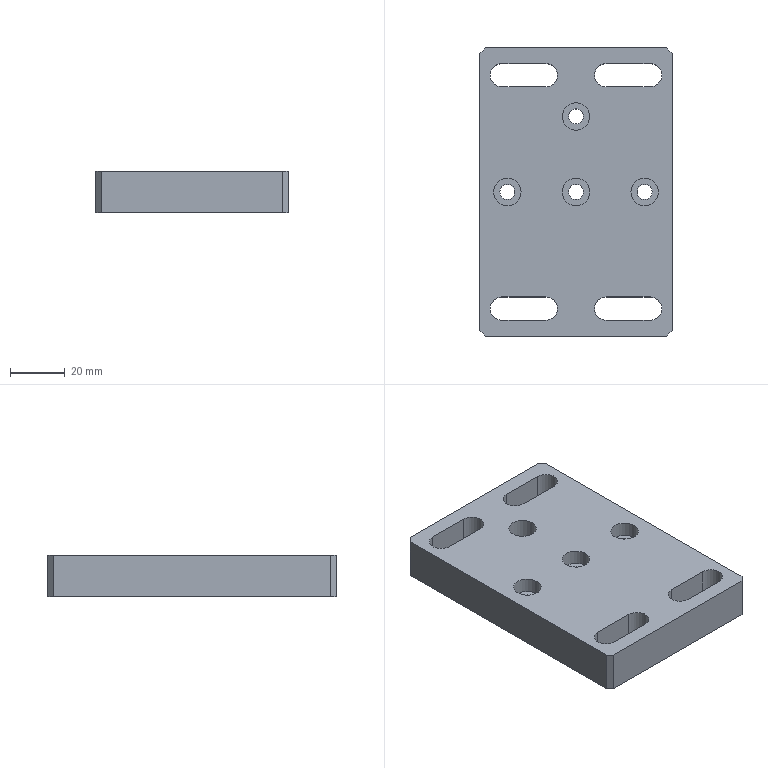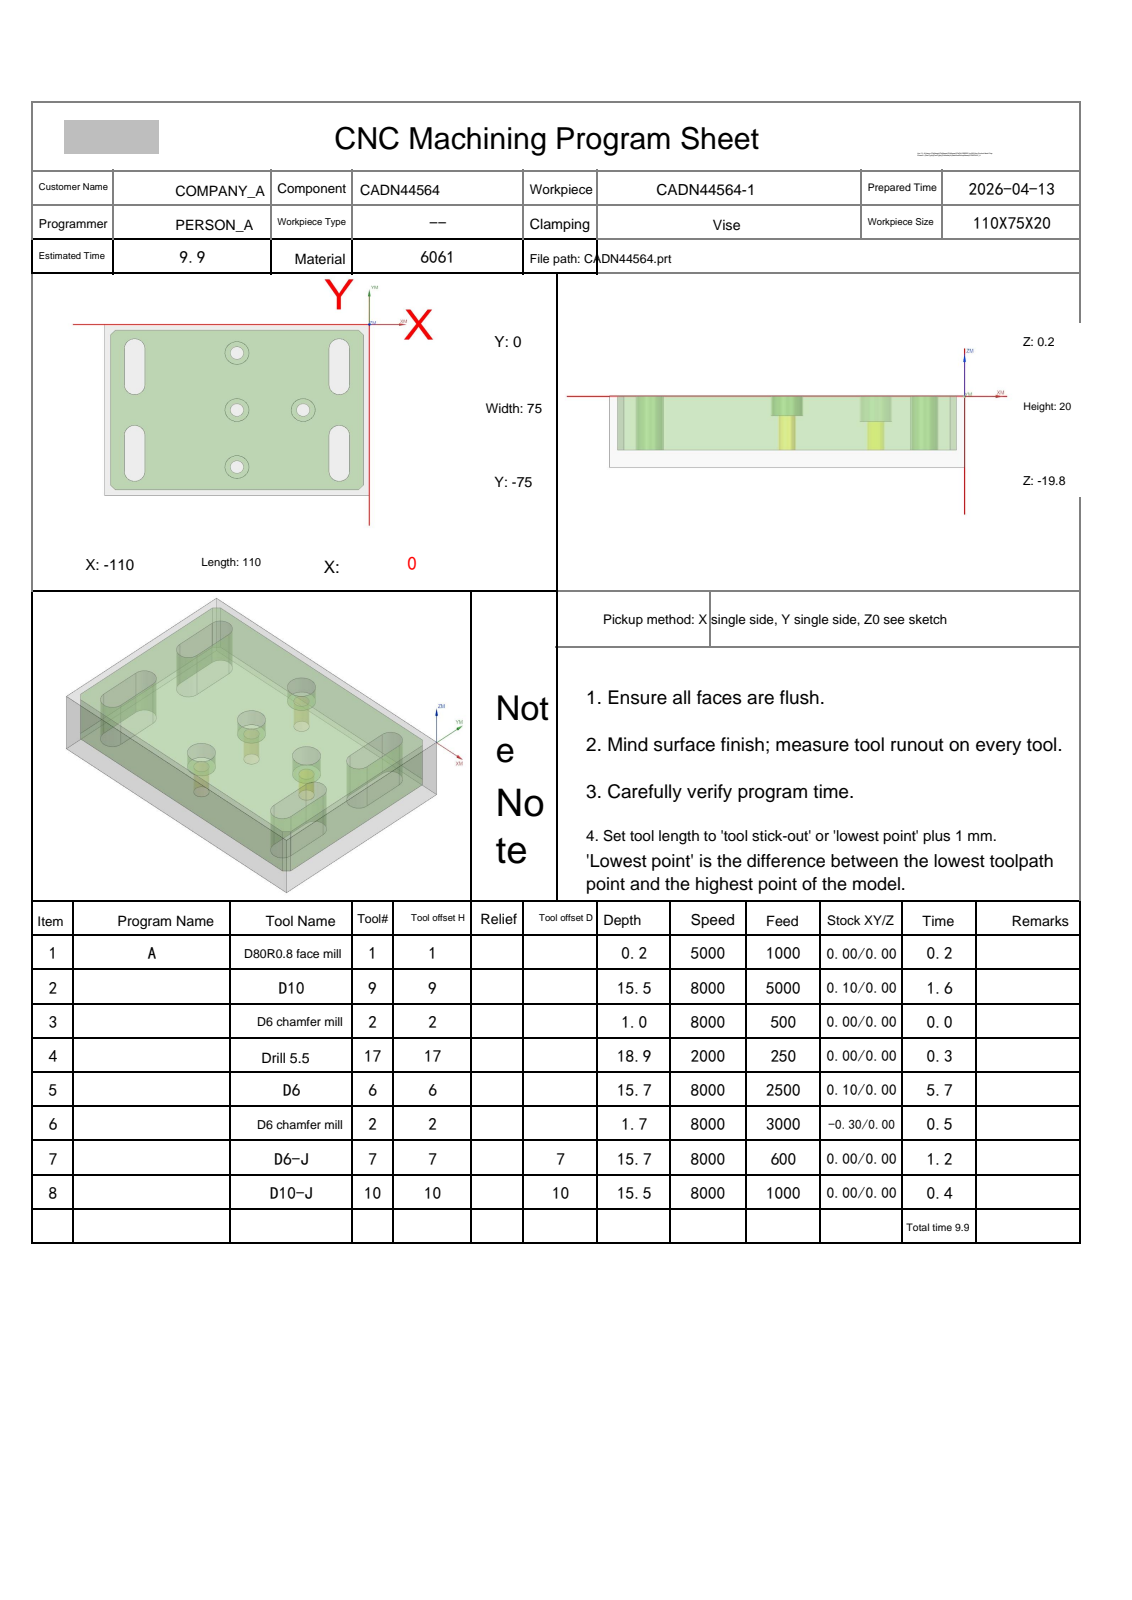NC program | NX | posted by the shop | part box 70 x 105 x 15 mm
Lines 2582 to 3183 of 3183:
N6 T02 M06
(D6 chamfer mill  D=6. R=0. H=02 ce=0.00 di=0.00)
G00 G90 G54 X-54.75 Y-74.628 M03 S8000
G43 H02 Z20.
M08
Z2.099
G01 Z-1.5 F3000.
G03 X-54.67 Y-74.328 I-.52 J.3
X-54.97 Y-73.808 I-.6 J0.0
G01 X-55. Y-73.8
X-105.5
X-105.754 Y-73.775
X-105.997 Y-73.701
X-106.222 Y-73.581
X-106.419 Y-73.419
X-108.419 Y-71.419
X-108.581 Y-71.222
X-108.701 Y-70.997
X-108.775 Y-70.754
X-108.8 Y-70.5
Y-4.5
X-108.775 Y-4.246
X-108.701 Y-4.003
X-108.581 Y-3.778
X-108.419 Y-3.581
X-106.419 Y-1.581
X-106.222 Y-1.419
X-105.997 Y-1.299
X-105.754 Y-1.225
X-105.5 Y-1.2
X-4.5
X-4.246 Y-1.225
X-4.003 Y-1.299
X-3.778 Y-1.419
X-3.581 Y-1.581
X-1.581 Y-3.581
X-1.419 Y-3.778
X-1.299 Y-4.003
X-1.225 Y-4.246
X-1.2 Y-4.5
Y-70.5
X-1.225 Y-70.754
X-1.299 Y-70.997
X-1.419 Y-71.222
X-1.581 Y-71.419
X-3.581 Y-73.419
X-3.778 Y-73.581
X-4.003 Y-73.701
X-4.246 Y-73.775
X-4.5 Y-73.8
X-55.
X-55.03 Y-73.808
G03 X-55.33 Y-74.328 I.3 J-.52
X-55.25 Y-74.628 I.6 J0.0
G01 Z2.099
G00 Z20.
X-95.378 Y-56.75
Z2.099
G01 Z-1.5
G03 X-95.078 Y-56.83 I.3 J.52
X-94.558 Y-56.53 I0.0 J.6
G01 X-94.55 Y-56.5
Y-48.5
G03 X-97.5 Y-45.55 I-2.95 J0.0
X-100.45 Y-48.5 I0.0 J-2.95
G01 Y-64.5
G03 X-97.5 Y-67.45 I2.95 J0.0
X-94.55 Y-64.5 I0.0 J2.95
G01 Y-56.5
X-94.558 Y-56.47
G03 X-95.078 Y-56.17 I-.52 J-.3
X-95.378 Y-56.25 I0.0 J-.6
G01 Z2.099
G00 Z20.
Y-18.75
Z2.099
G01 Z-1.5
G03 X-95.078 Y-18.83 I.3 J.52
X-94.558 Y-18.53 I0.0 J.6
G01 X-94.55 Y-18.5
Y-10.5
G03 X-97.5 Y-7.55 I-2.95 J0.0
X-100.45 Y-10.5 I0.0 J-2.95
G01 Y-26.5
G03 X-97.5 Y-29.45 I2.95 J0.0
X-94.55 Y-26.5 I0.0 J2.95
G01 Y-18.5
X-94.558 Y-18.47
G03 X-95.078 Y-18.17 I-.52 J-.3
X-95.378 Y-18.25 I0.0 J-.6
G01 Z2.099
G00 Z20.
X-14.622
Z2.099
G01 Z-1.5
G03 X-14.922 Y-18.17 I-.3 J-.52
X-15.442 Y-18.47 I0.0 J-.6
G01 X-15.45 Y-18.5
Y-26.5
G03 X-12.5 Y-29.45 I2.95 J0.0
X-9.55 Y-26.5 I0.0 J2.95
G01 Y-10.5
G03 X-12.5 Y-7.55 I-2.95 J0.0
X-15.45 Y-10.5 I0.0 J-2.95
G01 Y-18.5
X-15.442 Y-18.53
G03 X-14.922 Y-18.83 I.52 J.3
X-14.622 Y-18.75 I0.0 J.6
G01 Z2.099
G00 Z20.
Y-56.25
Z2.099
G01 Z-1.5
G03 X-14.922 Y-56.17 I-.3 J-.52
X-15.442 Y-56.47 I0.0 J-.6
G01 X-15.45 Y-56.5
Y-64.5
G03 X-12.5 Y-67.45 I2.95 J0.0
X-9.55 Y-64.5 I0.0 J2.95
G01 Y-48.5
G03 X-12.5 Y-45.55 I-2.95 J0.0
X-15.45 Y-48.5 I0.0 J-2.95
G01 Y-56.5
X-15.442 Y-56.53
G03 X-14.922 Y-56.83 I.52 J.3
X-14.622 Y-56.75 I0.0 J.6
G01 Z2.099
G00 Z20.
G00 G90 X-58.386 Y-9.846 M03 S8000
Z20.
Z2.5
G01 X-58.394 Y-9.855 Z2.495 F800.
X-58.644 Y-10.211 Z2.337
X-58.804 Y-10.489 Z2.22
X-58.988 Y-10.883 Z2.062
X-59.13 Y-11.293 Z1.904
X-59.231 Y-11.716 Z1.746
X-59.288 Y-12.146 Z1.588
X-59.302 Y-12.58 Z1.43
X-59.272 Y-13.014 Z1.272
X-59.199 Y-13.442 Z1.114
X-59.082 Y-13.86 Z.956
X-58.924 Y-14.265 Z.797
X-58.727 Y-14.652 Z.639
X-58.491 Y-15.016 Z.481
X-58.219 Y-15.355 Z.323
X-57.915 Y-15.665 Z.165
X-57.581 Y-15.943 Z.007
X-57.221 Y-16.186 Z-.151
X-56.838 Y-16.391 Z-.309
X-56.436 Y-16.556 Z-.467
X-56.02 Y-16.68 Z-.625
X-55.593 Y-16.762 Z-.783
X-55.161 Y-16.8 Z-.942
X-55. Z-1.
G03 X-50.7 Y-12.5 I0.0 J4.3
X-55. Y-8.2 I-4.3 J0.0
X-59.3 Y-12.5 I0.0 J-4.3
X-55. Y-16.8 I4.3 J0.0
X-54.501 Y-16.771 I0.0 J4.3
G01 Z1.5
G00 Z20.
X-58.386 Y-34.846
Z2.5
G01 X-58.394 Y-34.855 Z2.495
X-58.644 Y-35.211 Z2.337
X-58.804 Y-35.489 Z2.22
X-58.988 Y-35.883 Z2.062
X-59.13 Y-36.293 Z1.904
X-59.231 Y-36.716 Z1.746
X-59.288 Y-37.146 Z1.588
X-59.302 Y-37.58 Z1.43
X-59.272 Y-38.014 Z1.272
X-59.199 Y-38.442 Z1.114
X-59.082 Y-38.86 Z.956
X-58.924 Y-39.265 Z.797
X-58.727 Y-39.652 Z.639
X-58.491 Y-40.016 Z.481
X-58.219 Y-40.355 Z.323
X-57.915 Y-40.665 Z.165
X-57.581 Y-40.943 Z.007
X-57.221 Y-41.186 Z-.151
X-56.838 Y-41.391 Z-.309
X-56.436 Y-41.556 Z-.467
X-56.02 Y-41.68 Z-.625
X-55.593 Y-41.762 Z-.783
X-55.161 Y-41.8 Z-.942
X-55. Z-1.
G03 X-50.7 Y-37.5 I0.0 J4.3
X-55. Y-33.2 I-4.3 J0.0
X-59.3 Y-37.5 I0.0 J-4.3
X-55. Y-41.8 I4.3 J0.0
X-54.501 Y-41.771 I0.0 J4.3
G01 Z1.5
G00 Z20.
X-58.386 Y-59.846
Z2.5
G01 X-58.394 Y-59.855 Z2.495
X-58.644 Y-60.211 Z2.337
X-58.804 Y-60.489 Z2.22
X-58.988 Y-60.883 Z2.062
X-59.13 Y-61.293 Z1.904
X-59.231 Y-61.716 Z1.746
X-59.288 Y-62.146 Z1.588
X-59.302 Y-62.58 Z1.43
X-59.272 Y-63.014 Z1.272
X-59.199 Y-63.442 Z1.114
X-59.082 Y-63.86 Z.956
X-58.924 Y-64.265 Z.797
X-58.727 Y-64.652 Z.639
X-58.491 Y-65.016 Z.481
X-58.219 Y-65.355 Z.323
X-57.915 Y-65.665 Z.165
X-57.581 Y-65.943 Z.007
X-57.221 Y-66.186 Z-.151
X-56.838 Y-66.391 Z-.309
X-56.436 Y-66.556 Z-.467
X-56.02 Y-66.68 Z-.625
X-55.593 Y-66.762 Z-.783
X-55.161 Y-66.8 Z-.942
X-55. Z-1.
G03 X-50.7 Y-62.5 I0.0 J4.3
X-55. Y-58.2 I-4.3 J0.0
X-59.3 Y-62.5 I0.0 J-4.3
X-55. Y-66.8 I4.3 J0.0
X-54.501 Y-66.771 I0.0 J4.3
G01 Z1.5
G00 Z20.
X-30.886 Y-34.846
Z2.5
G01 X-30.894 Y-34.855 Z2.495
X-31.144 Y-35.211 Z2.337
X-31.304 Y-35.489 Z2.22
X-31.488 Y-35.883 Z2.062
X-31.63 Y-36.293 Z1.904
X-31.731 Y-36.716 Z1.746
X-31.788 Y-37.146 Z1.588
X-31.802 Y-37.58 Z1.43
X-31.772 Y-38.014 Z1.272
X-31.699 Y-38.442 Z1.114
X-31.582 Y-38.86 Z.956
X-31.424 Y-39.265 Z.797
X-31.227 Y-39.652 Z.639
X-30.991 Y-40.016 Z.481
X-30.719 Y-40.355 Z.323
X-30.415 Y-40.665 Z.165
X-30.081 Y-40.943 Z.007
X-29.721 Y-41.186 Z-.151
X-29.338 Y-41.391 Z-.309
X-28.936 Y-41.556 Z-.467
X-28.52 Y-41.68 Z-.625
X-28.093 Y-41.762 Z-.783
X-27.661 Y-41.8 Z-.942
X-27.5 Z-1.
G03 X-23.2 Y-37.5 I0.0 J4.3
X-27.5 Y-33.2 I-4.3 J0.0
X-31.8 Y-37.5 I0.0 J-4.3
X-27.5 Y-41.8 I4.3 J0.0
X-27.001 Y-41.771 I0.0 J4.3
G01 Z1.5
G00 Z20.
G91 G28 Z0.0
M05
M09
G91 G28 Z0.0
M01
N7 T07 M06
(D6-J  D=6. R=0. H=07 ce=0.00 di=0.00)
G00 G90 G54 X-27.5 Y-37.5 M03 S8000
G43 H07 Z20.
M08
Z0.0
G41 D07
G01 X-27.696 Y-37.54 F500.
G03 X-28.49 Y-38.51 I.196 J-.97
X-27.5 Y-39.5 I.99 J0.0
X-27.5 Y-39.5 Z-5. I0.0 J2.
X-26.324 Y-35.882 Z-7. I0.0 J2.
X-27.5 Y-35.5 I-1.176 J-1.618
X-29.5 Y-37.5 I0.0 J-2.
X-27.5 Y-39.5 I2. J0.0
X-25.5 Y-37.5 I0.0 J2.
X-26.324 Y-35.882 I-2. J0.0
X-26.906 Y-35.693 I-.582 J-.801
X-27.896 Y-36.683 I0.0 J-.99
X-27.635 Y-37.353 I.99 J0.0
G01 G40 X-27.5 Y-37.5
G00 Z20.
G00 G90 X-55. Y-62.5 M03 S8000
Z20.
Z0.0
G41 D07
G01 X-55.196 Y-62.54 F500.
G03 X-55.99 Y-63.51 I.196 J-.97
X-55. Y-64.5 I.99 J0.0
X-55. Y-64.5 Z-5. I0.0 J2.
X-54.036 Y-64.253 Z-5.4 I0.0 J2.
X-53. Y-62.5 I-.964 J1.753
X-55. Y-60.5 I-2. J0.0
X-57. Y-62.5 I0.0 J-2.
X-55. Y-64.5 I2. J0.0
X-54.036 Y-64.253 I0.0 J2.
X-53.523 Y-63.385 I-.477 J.868
X-54.513 Y-62.395 I-.99 J0.0
X-54.809 Y-62.44 I0.0 J-.99
G01 G40 X-55. Y-62.5
G00 Z20.
Y-37.5
Z0.0
G41 D07
G01 X-55.196 Y-37.54
G03 X-55.99 Y-38.51 I.196 J-.97
X-55. Y-39.5 I.99 J0.0
X-55. Y-39.5 Z-5. I0.0 J2.
X-54.036 Y-39.253 Z-5.4 I0.0 J2.
X-53. Y-37.5 I-.964 J1.753
X-55. Y-35.5 I-2. J0.0
X-57. Y-37.5 I0.0 J-2.
X-55. Y-39.5 I2. J0.0
X-54.036 Y-39.253 I0.0 J2.
X-53.523 Y-38.385 I-.477 J.868
X-54.513 Y-37.395 I-.99 J0.0
X-54.809 Y-37.44 I0.0 J-.99
G01 G40 X-55. Y-37.5
G00 Z20.
Y-12.5
Z0.0
G41 D07
G01 X-55.196 Y-12.54
G03 X-55.99 Y-13.51 I.196 J-.97
X-55. Y-14.5 I.99 J0.0
X-55. Y-14.5 Z-5. I0.0 J2.
X-54.036 Y-14.253 Z-5.4 I0.0 J2.
X-53. Y-12.5 I-.964 J1.753
X-55. Y-10.5 I-2. J0.0
X-57. Y-12.5 I0.0 J-2.
X-55. Y-14.5 I2. J0.0
X-54.036 Y-14.253 I0.0 J2.
X-53.523 Y-13.385 I-.477 J.868
X-54.513 Y-12.395 I-.99 J0.0
X-54.809 Y-12.44 I0.0 J-.99
G01 G40 X-55. Y-12.5
G00 Z20.
G00 G90 X-11.5 Y-18.7 M03 S6000
Z20.
Z-4.667
G01 Z-5.167 F600.
G41 D07
X-11.45
G03 X-11.25 Y-18.5 I0.0 J.2
G01 Y-10.5
G03 X-12.5 Y-9.25 I-1.25 J0.0
X-13.75 Y-10.5 I0.0 J-1.25
G01 Y-26.5
G03 X-12.5 Y-27.75 I1.25 J0.0
X-11.25 Y-26.5 I0.0 J1.25
G01 Y-18.5
Y-18.
G03 X-11.45 Y-17.8 I-.2 J0.0
G01 G40 X-11.5
Z-4.667
G00 Z1.
Y-18.7
Z-9.833
G01 Z-10.333
G41 D07
X-11.45
G03 X-11.25 Y-18.5 I0.0 J.2
G01 Y-10.5
G03 X-12.5 Y-9.25 I-1.25 J0.0
X-13.75 Y-10.5 I0.0 J-1.25
G01 Y-26.5
G03 X-12.5 Y-27.75 I1.25 J0.0
X-11.25 Y-26.5 I0.0 J1.25
G01 Y-18.5
Y-18.
G03 X-11.45 Y-17.8 I-.2 J0.0
G01 G40 X-11.5
Z-9.833
G00 Z-4.167
Y-18.7
Z-15.
G01 Z-15.5
G41 D07
X-11.45
G03 X-11.25 Y-18.5 I0.0 J.2
G01 Y-10.5
G03 X-12.5 Y-9.25 I-1.25 J0.0
X-13.75 Y-10.5 I0.0 J-1.25
G01 Y-26.5
G03 X-12.5 Y-27.75 I1.25 J0.0
X-11.25 Y-26.5 I0.0 J1.25
G01 Y-18.5
Y-18.
G03 X-11.45 Y-17.8 I-.2 J0.0
G01 G40 X-11.5
Z-15.
G00 Z20.
Y-56.7
Z-4.667
G01 Z-5.167
G41 D07
X-11.45
G03 X-11.25 Y-56.5 I0.0 J.2
G01 Y-48.5
G03 X-12.5 Y-47.25 I-1.25 J0.0
X-13.75 Y-48.5 I0.0 J-1.25
G01 Y-64.5
G03 X-12.5 Y-65.75 I1.25 J0.0
X-11.25 Y-64.5 I0.0 J1.25
G01 Y-56.5
Y-56.
G03 X-11.45 Y-55.8 I-.2 J0.0
G01 G40 X-11.5
Z-4.667
G00 Z1.
Y-56.7
Z-9.833
G01 Z-10.333
G41 D07
X-11.45
G03 X-11.25 Y-56.5 I0.0 J.2
G01 Y-48.5
G03 X-12.5 Y-47.25 I-1.25 J0.0
X-13.75 Y-48.5 I0.0 J-1.25
G01 Y-64.5
G03 X-12.5 Y-65.75 I1.25 J0.0
X-11.25 Y-64.5 I0.0 J1.25
G01 Y-56.5
Y-56.
G03 X-11.45 Y-55.8 I-.2 J0.0
G01 G40 X-11.5
Z-9.833
G00 Z-4.167
Y-56.7
Z-15.
G01 Z-15.5
G41 D07
X-11.45
G03 X-11.25 Y-56.5 I0.0 J.2
G01 Y-48.5
G03 X-12.5 Y-47.25 I-1.25 J0.0
X-13.75 Y-48.5 I0.0 J-1.25
G01 Y-64.5
G03 X-12.5 Y-65.75 I1.25 J0.0
X-11.25 Y-64.5 I0.0 J1.25
G01 Y-56.5
Y-56.
G03 X-11.45 Y-55.8 I-.2 J0.0
G01 G40 X-11.5
Z-15.
G00 Z20.
X-98.5 Y-56.3
Z-4.667
G01 Z-5.167
G41 D07
X-98.55
G03 X-98.75 Y-56.5 I0.0 J-.2
G01 Y-64.5
G03 X-97.5 Y-65.75 I1.25 J0.0
X-96.25 Y-64.5 I0.0 J1.25
G01 Y-48.5
G03 X-97.5 Y-47.25 I-1.25 J0.0
X-98.75 Y-48.5 I0.0 J-1.25
G01 Y-56.5
Y-57.
G03 X-98.55 Y-57.2 I.2 J0.0
G01 G40 X-98.5
Z-4.667
G00 Z1.
Y-56.3
Z-9.833
G01 Z-10.333
G41 D07
X-98.55
G03 X-98.75 Y-56.5 I0.0 J-.2
G01 Y-64.5
G03 X-97.5 Y-65.75 I1.25 J0.0
X-96.25 Y-64.5 I0.0 J1.25
G01 Y-48.5
G03 X-97.5 Y-47.25 I-1.25 J0.0
X-98.75 Y-48.5 I0.0 J-1.25
G01 Y-56.5
Y-57.
G03 X-98.55 Y-57.2 I.2 J0.0
G01 G40 X-98.5
Z-9.833
G00 Z-4.167
Y-56.3
Z-15.
G01 Z-15.5
G41 D07
X-98.55
G03 X-98.75 Y-56.5 I0.0 J-.2
G01 Y-64.5
G03 X-97.5 Y-65.75 I1.25 J0.0
X-96.25 Y-64.5 I0.0 J1.25
G01 Y-48.5
G03 X-97.5 Y-47.25 I-1.25 J0.0
X-98.75 Y-48.5 I0.0 J-1.25
G01 Y-56.5
Y-57.
G03 X-98.55 Y-57.2 I.2 J0.0
G01 G40 X-98.5
Z-15.
G00 Z20.
Y-18.3
Z-4.667
G01 Z-5.167
G41 D07
X-98.55
G03 X-98.75 Y-18.5 I0.0 J-.2
G01 Y-26.5
G03 X-97.5 Y-27.75 I1.25 J0.0
X-96.25 Y-26.5 I0.0 J1.25
G01 Y-10.5
G03 X-97.5 Y-9.25 I-1.25 J0.0
X-98.75 Y-10.5 I0.0 J-1.25
G01 Y-18.5
Y-19.
G03 X-98.55 Y-19.2 I.2 J0.0
G01 G40 X-98.5
Z-4.667
G00 Z1.
Y-18.3
Z-9.833
G01 Z-10.333
G41 D07
X-98.55
G03 X-98.75 Y-18.5 I0.0 J-.2
G01 Y-26.5
G03 X-97.5 Y-27.75 I1.25 J0.0
X-96.25 Y-26.5 I0.0 J1.25
G01 Y-10.5
G03 X-97.5 Y-9.25 I-1.25 J0.0
X-98.75 Y-10.5 I0.0 J-1.25
G01 Y-18.5
Y-19.
G03 X-98.55 Y-19.2 I.2 J0.0
G01 G40 X-98.5
Z-9.833
G00 Z-4.167
Y-18.3
Z-15.
G01 Z-15.5
G41 D07
X-98.55
G03 X-98.75 Y-18.5 I0.0 J-.2
G01 Y-26.5
G03 X-97.5 Y-27.75 I1.25 J0.0
X-96.25 Y-26.5 I0.0 J1.25
G01 Y-10.5
G03 X-97.5 Y-9.25 I-1.25 J0.0
X-98.75 Y-10.5 I0.0 J-1.25
G01 Y-18.5
Y-19.
G03 X-98.55 Y-19.2 I.2 J0.0
G01 G40 X-98.5
Z-15.
G00 Z20.
G91 G28 Z0.0
M05
M09
G91 G28 Z0.0
M01
N8 T10 M06
(D10-J  D=10. R=0. H=10 ce=0.00 di=0.00)
G00 G90 G54 X-3.487 Y-78.616 M03 S8000
G43 H10 Z20.
M08
Z-14.8
G01 Z-15.3 F1000.
G41 D10
X-3.503 Y-78.417
G03 X-4.5 Y-77.5 I-.997 J-.083
G01 X-105.5
G02 X-109.036 Y-76.036 I0.0 J5.
G01 X-111.036 Y-74.036
G02 X-112.5 Y-70.5 I3.536 J3.536
G01 Y-4.5
G02 X-111.036 Y-.964 I5. J0.0
G01 X-109.036 Y1.036
G02 X-105.5 Y2.5 I3.536 J-3.536
G01 X-4.5
G02 X-.964 Y1.036 I0.0 J-5.
G01 X1.036 Y-.964
G02 X2.5 Y-4.5 I-3.536 J-3.536
G01 Y-70.5
G02 X1.036 Y-74.036 I-5. J0.0
G01 X-.964 Y-76.036
G02 X-4.5 Y-77.5 I-3.536 J3.536
G01 X-5.
G03 X-6. Y-78.5 I0.0 J-1.
G01 G40 Y-78.7
Z-14.8
G00 Z20.
M05
M09
G91 G28 Z0.0
G91 G28 Y0.0
M30
%